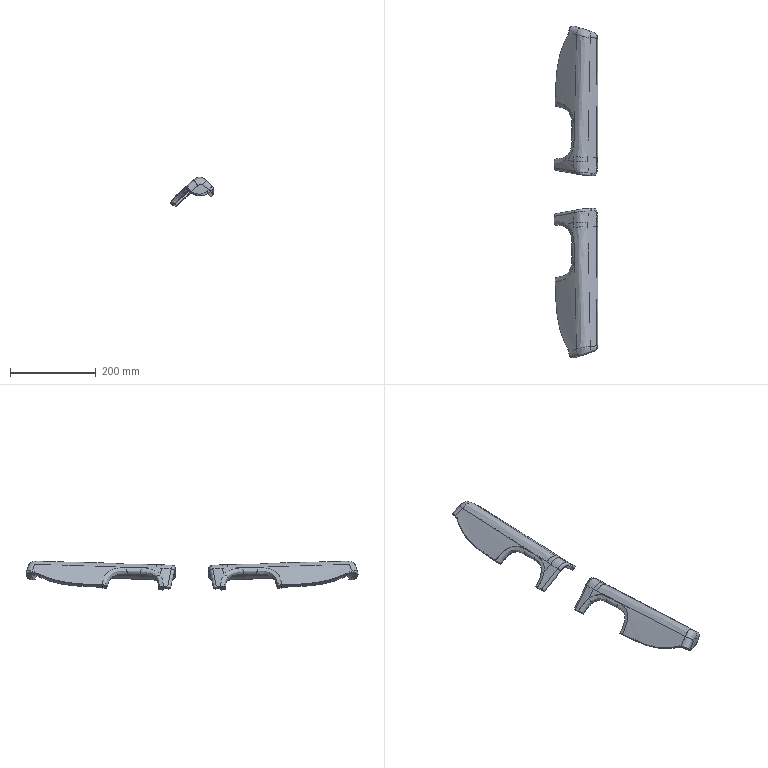Part | STEP file | L0193017AA ARMREST FRT DR MANUAL!SKIN VINYL ARMREST FRT DR MANUAL | 2 solids | 638 faces | box 102.007 x 773.524 x 69.683 mm | volume 142279 mm3 | spline 620 | plane 18